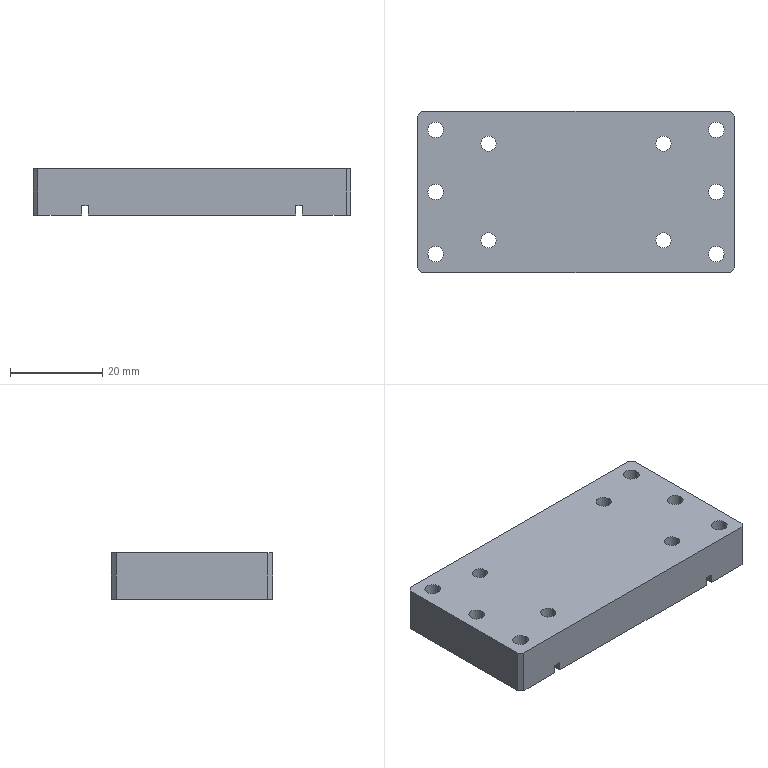Part | STEP file | 11-FG-S02411 | 1 solid | 56 faces | box 69 x 35 x 10 mm | volume 22541 mm3 | cylinder 32 | plane 24 | commonest cylinder face diameters 3.4 x12 6.5 x12 3.3 x8